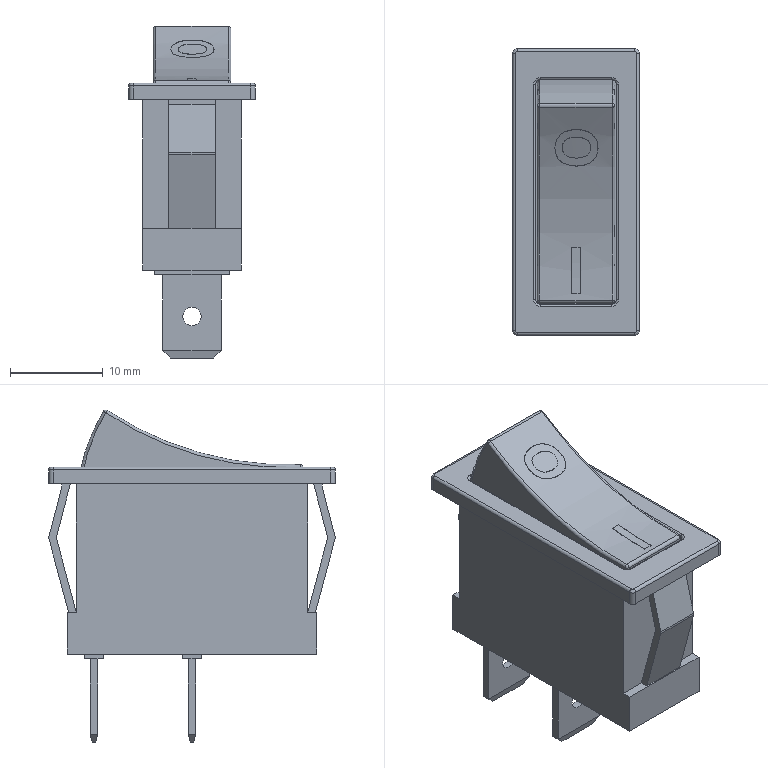Part | STEP file | Rocker switch KCD3-50A | 1 solid | 118 faces | box 13.7 x 31 x 35.877 mm | volume 6384 mm3 | plane 69 | cylinder 31 | torus 8 | spline 6 | sphere 4 | commonest cylinder face diameters 1 x12 0.6 x8 0.44 x4 2 x2 70 x2 70.02 x2